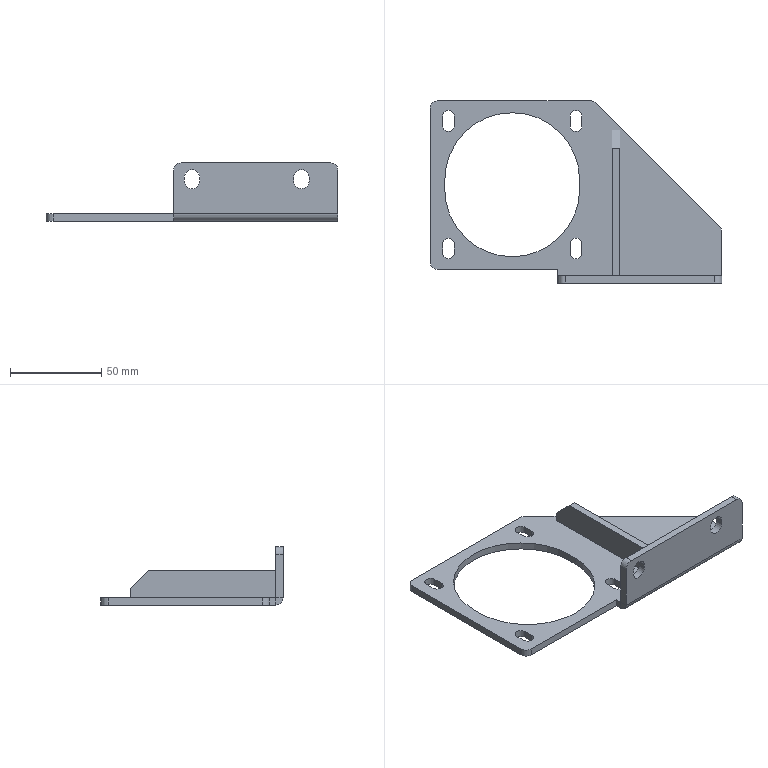Part | STEP file | 2 solids | 60 faces | box 160 x 100 x 32 mm | volume 46086 mm3 | plane 36 | cylinder 24 | commonest cylinder face diameters 6.5 x8 8 x6 8.4 x6 74 x2 0.2 x1 8.2 x1